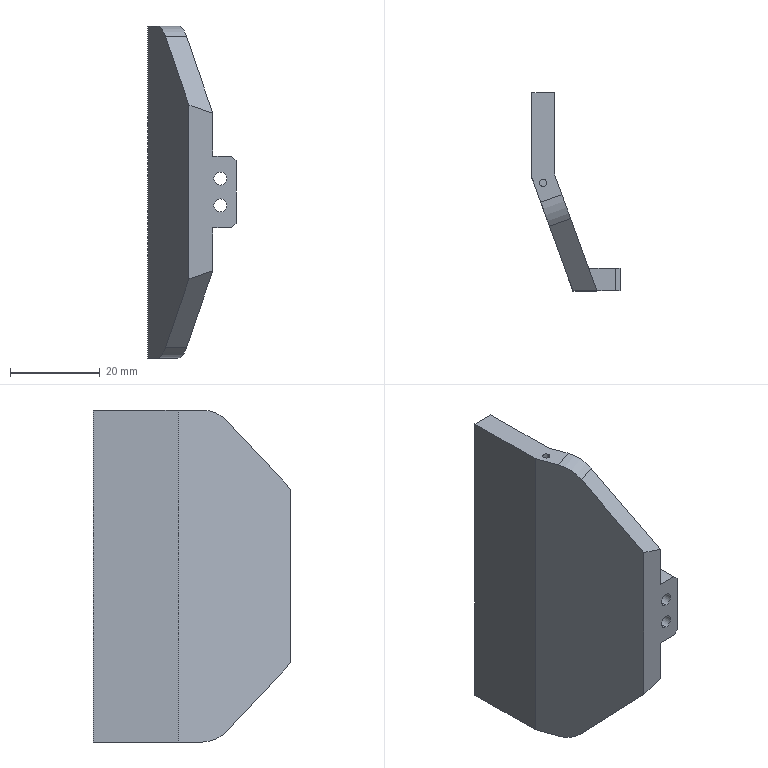NC program | NX | posted with a generic post | part box 19.643 x 44.061 x 74 mm
Lines 2592 to 2613 of 2613:
(FLOOR_FACING_2 , TOOL : D8精光)
N5182 T03 M6
N5184 G54
N5186 G17 G0 G90 X-44. Y-27.118 B0. C0. S4500 M3
N5188 G43 Z30. H3
N5190 Z3.
N5192 G94 G1 Z0. F800.
N5194 X-41.
N5196 X41.
N5198 Y-31.433
N5200 X-41.
N5202 Y-35.747
N5204 X41.
N5206 Y-40.061
N5208 X-41.
N5210 X-47.
N5212 Z3.
N5214 G0 Z30.
N5216 M5
N5218 M2